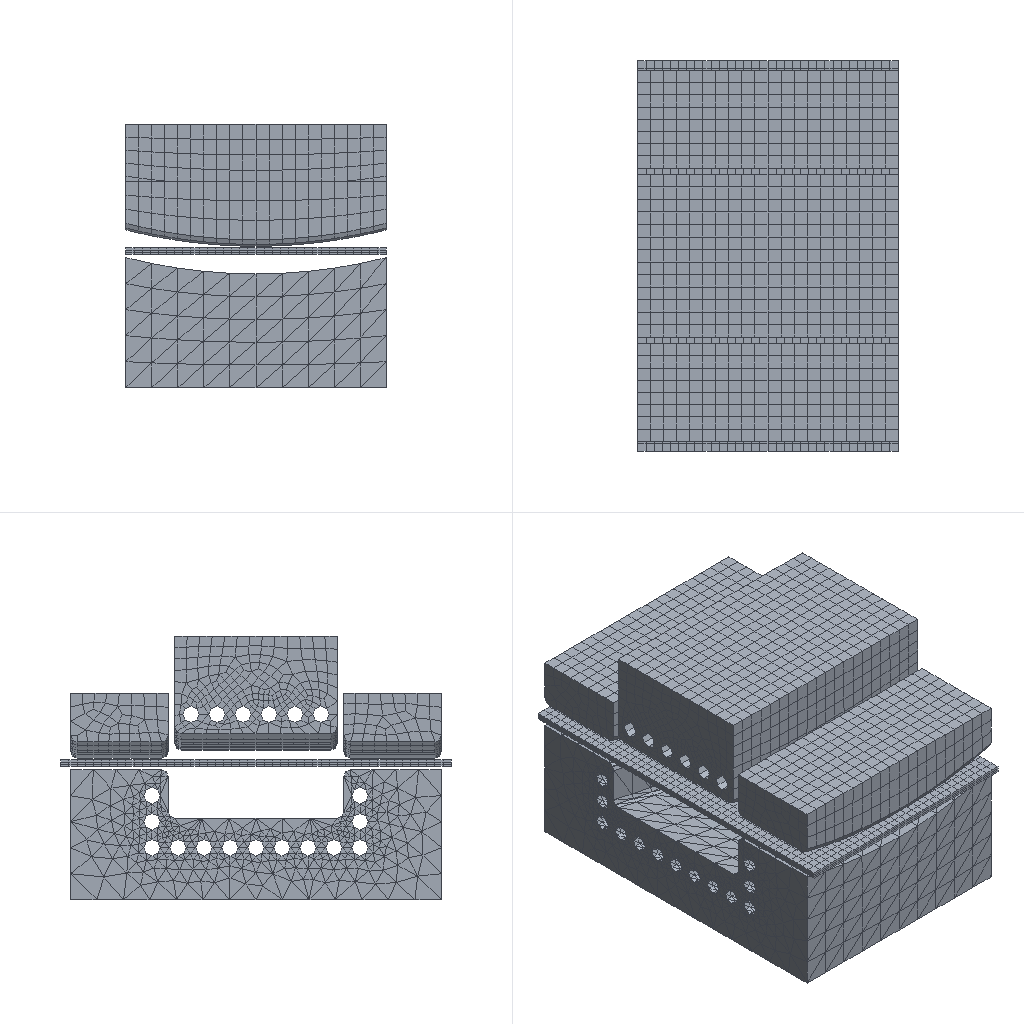Simulation study | abaqus
Set-up summary:
category,name,step,type,value,unit,region
solver,abaqus
solver,version,,,Abaqus/Explicit 2020
units,not stated in the deck,,not stated
analysis,deck,,dynamic temperature-displacement,dynamic temperature-displacement
load_step,Step-1,Step-1,dynamic temperature-displacement
load_step,requested,,,1
mesh,nodes,,,24140
mesh,elements,,,54890
element_type,C3D4,,solid,44042
element_type,C3D8R,,solid,6240
element_type,C3D8RT,,solid,4608
load,load commands in deck,,count,4
bc,support commands in deck,,count,15
material,MATERIAL-1,,in results
material,MATERIAL-RIGID,,in results
check,setup vs results,,match,"per instance, exact: element labels, types and connectivity; labels of the nodes the elements use; coordinates not compared"
Abaqus input file, long lists of numbers shortened:
*Heading
** Job name: Job-2 Model name: Model-1
** Generated by: Abaqus/CAE 2020
*Preprint, echo=NO, model=NO, history=NO, contact=NO
**
** PARTS
**
*Part, name=zhuangpeitu-1
*Node
      1,         -40.,          60.,           1.
      2,         -40.,         57.5,           1.
** (6466 more lines like these left out)
*Element, type=C3D8RT
   1,  197,  198,  247,  246,    1,    2,   51,   50
   2,  198,  199,  248,  247,    2,    3,   52,   51
** (4606 more lines like these left out)
*Nset, nset=Set-3, generate
    1,  6468,     1
*Elset, elset=Set-3, generate
    1,  4608,     1
*Nset, nset=tt, generate
    1,  6468,     1
** Section: Section-1
*Solid Section, elset=Set-3, material=Material-1
,
*End Part
**
*Part, name=zhuangpeitu-2
*Node
      1,         -40.,          32.,        -13.5
      2,         -40.,           8.,        -21.5
** (9669 more lines like these left out)
*Element, type=C3D4
    1, 5348, 5349, 5350, 5351
    2, 5348, 5352, 5349, 5351
** (44040 more lines like these left out)
*Nset, nset=Set-10, generate
    1,  9671,     1
*Elset, elset=Set-10, generate
     1,  44042,      1
** Section: Section-2
*Solid Section, elset=Set-10, material=Material-rigid
,
*End Part
**
*Part, name=zhuangpeitu-3
*Node
      1,         -40.,    18.232,    20.268
      2,         -40.,         17.5,         18.5
** (5689 more lines like these left out)
*Element, type=C3D8R
   1,  152,  155,  158,  257,  423,  426,  429,  528
   2,  135,   93,   48,   47,  406,  364,  319,  318
** (4598 more lines like these left out)
*Nset, nset=Set-2, generate
    1,  5691,     1
*Elset, elset=Set-2, generate
    1,  4600,     1
** Section: Section-2
*Solid Section, elset=Set-2, material=Material-rigid
,
*End Part
**
*Part, name=zhuangpeitu-4
*Node
      1,         -40.,          55.,          10.
      2,         -40.,          29.,          10.
** (1174 more lines like these left out)
*Element, type=C3D8R
  1,   22,   38,   37,   21,   78,   94,   93,   77
  2,    2,   33,    4,    3,   58,   89,   60,   59
** (838 more lines like these left out)
*Nset, nset=Set-2, generate
    1,  1176,     1
*Elset, elset=Set-2, generate
   1,  840,    1
** Section: Section-2
*Solid Section, elset=Set-2, material=Material-rigid
,
*End Part
**
*Part, name=zhuangpeitu-5
*Node
      1,         -40.,         -27.,          25.
      2,         -40.,         -27.,   12.064
** (1132 more lines like these left out)
*Element, type=C3D8R
  1,   54,   17,    4,   53,  108,   71,   58,  107
  2,   23,   37,   38,   24,   77,   91,   92,   78
** (798 more lines like these left out)
*Nset, nset=Set-2, generate
    1,  1134,     1
*Elset, elset=Set-2, generate
   1,  800,    1
** Section: Section-2
*Solid Section, elset=Set-2, material=Material-rigid
,
*End Part
**
**
** ASSEMBLY
**
*Assembly, name=Assembly
**
*Instance, name=zhuangpeitu-1-1, part=zhuangpeitu-1
*End Instance
**
*Instance, name=zhuangpeitu-2-1, part=zhuangpeitu-2
*End Instance
**
*Instance, name=zhuangpeitu-3-1, part=zhuangpeitu-3
          0.,           0.,         -1.5
*End Instance
**
*Instance, name=zhuangpeitu-4-1, part=zhuangpeitu-4
          0.,           0.,         -1.5
*End Instance
**
*Instance, name=zhuangpeitu-5-1, part=zhuangpeitu-5
          0.,           0.,         -1.5
*End Instance
**
*Node
      1,          40.,         -42.,         23.5
*Node
      2,          40.,          42.,         23.5
*Node
      3,          40.,           0.,          41.
*Node
      4,          40.,           0.,         -40.
*Nset, nset=Set-9, instance=zhuangpeitu-1-1, generate
    1,  6468,     1
*Nset, nset=Set-9, instance=zhuangpeitu-2-1, generate
    1,  9671,     1
*Nset, nset=Set-9, instance=zhuangpeitu-4-1, generate
    1,  1176,     1
*Nset, nset=Set-9, instance=zhuangpeitu-3-1, generate
    1,  5691,     1
*Nset, nset=Set-9, instance=zhuangpeitu-5-1, generate
    1,  1134,     1
*Elset, elset=Set-9, instance=zhuangpeitu-1-1, generate
    1,  4608,     1
*Elset, elset=Set-9, instance=zhuangpeitu-2-1, generate
     1,  44042,      1
*Elset, elset=Set-9, instance=zhuangpeitu-4-1, generate
   1,  840,    1
*Elset, elset=Set-9, instance=zhuangpeitu-3-1, generate
    1,  4600,     1
*Elset, elset=Set-9, instance=zhuangpeitu-5-1, generate
   1,  800,    1
*Nset, nset=Set-10
 1, 2
*Nset, nset=Set-11
 3,
*Nset, nset=Set-12
 4,
*Nset, nset=Set-13, instance=zhuangpeitu-1-1, generate
    1,  6468,     1
*Elset, elset=Set-13, instance=zhuangpeitu-1-1, generate
    1,  4608,     1
*Nset, nset=Set-14, instance=zhuangpeitu-1-1
    1,   49,   50,   98,   99,  147,  148,  196,  197,  245,  246,  294,  295,  343,  344,  392
  393,  441,  442,  490,  491,  539,  540,  588,  589,  637,  638,  686,  687,  735,  736,  784
** (15 more lines like these left out)
*Elset, elset=Set-14, instance=zhuangpeitu-1-1
    1,   48,   49,   96,   97,  144,  145,  192,  193,  240,  241,  288,  289,  336,  337,  384
  385,  432,  433,  480,  481,  528,  529,  576,  577,  624,  625,  672,  673,  720,  721,  768
** (10 more lines like these left out)
*Nset, nset=Set-15, instance=zhuangpeitu-1-1
    1,    2,    3,    4,    5,    6,    7,    8,    9,   10,   11,   12,   13,   14,   15,   16
   17,   18,   19,   20,   21,   22,   23,   24,   25,   26,   27,   28,   29,   30,   31,   32
** (23 more lines like these left out)
*Elset, elset=Set-15, instance=zhuangpeitu-1-1
    1,    2,    3,    4,    5,    6,    7,    8,    9,   10,   11,   12,   13,   14,   15,   16
   17,   18,   19,   20,   21,   22,   23,   24,   25,   26,   27,   28,   29,   30,   31,   32
** (16 more lines like these left out)
*Nset, nset=b_Set-1, instance=zhuangpeitu-3-1, generate
    1,  5691,     1
*Elset, elset=b_Set-1, instance=zhuangpeitu-3-1, generate
    1,  4600,     1
*Nset, nset=b_Set-3, instance=zhuangpeitu-5-1, generate
    1,  1134,     1
*Elset, elset=b_Set-3, instance=zhuangpeitu-5-1, generate
   1,  800,    1
*Nset, nset=b_Set-5, instance=zhuangpeitu-4-1, generate
    1,  1176,     1
*Elset, elset=b_Set-5, instance=zhuangpeitu-4-1, generate
   1,  840,    1
*Nset, nset=b_Set-7, instance=zhuangpeitu-2-1, generate
    1,  9671,     1
*Elset, elset=b_Set-7, instance=zhuangpeitu-2-1, generate
     1,  44042,      1
*Nset, nset=_PickedSet17, internal
 3,
*Nset, nset=_PickedSet19, internal
 1,
*Nset, nset=_PickedSet21, internal
 2,
*Nset, nset=_PickedSet23, internal
 4,
*Elset, elset=_Surf-7_S1, internal, instance=zhuangpeitu-1-1, generate
 4465,  4608,     1
*Elset, elset=_Surf-7_S4, internal, instance=zhuangpeitu-1-1, generate
   48,  4608,    48
*Elset, elset=_Surf-7_S2, internal, instance=zhuangpeitu-1-1, generate
   1,  144,    1
*Elset, elset=_Surf-7_S6, internal, instance=zhuangpeitu-1-1, generate
    1,  4561,    48
*Elset, elset=_Surf-7_S5, internal, instance=zhuangpeitu-1-1
   97,   98,   99,  100,  101,  102,  103,  104,  105,  106,  107,  108,  109,  110,  111,  112
  113,  114,  115,  116,  117,  118,  119,  120,  121,  122,  123,  124,  125,  126,  127,  128
** (94 more lines like these left out)
*Elset, elset=_Surf-7_S3, internal, instance=zhuangpeitu-1-1
    1,    2,    3,    4,    5,    6,    7,    8,    9,   10,   11,   12,   13,   14,   15,   16
   17,   18,   19,   20,   21,   22,   23,   24,   25,   26,   27,   28,   29,   30,   31,   32
** (94 more lines like these left out)
*Surface, type=ELEMENT, name=Surf-7
_Surf-7_S1, S1
_Surf-7_S4, S4
_Surf-7_S2, S2
_Surf-7_S6, S6
_Surf-7_S5, S5
_Surf-7_S3, S3
*Elset, elset=_Surf-8_S1, internal, instance=zhuangpeitu-1-1, generate
 4465,  4608,     1
*Elset, elset=_Surf-8_S2, internal, instance=zhuangpeitu-1-1, generate
   1,  144,    1
*Elset, elset=_Surf-8_S5, internal, instance=zhuangpeitu-1-1
   97,   98,   99,  100,  101,  102,  103,  104,  105,  106,  107,  108,  109,  110,  111,  112
  113,  114,  115,  116,  117,  118,  119,  120,  121,  122,  123,  124,  125,  126,  127,  128
** (94 more lines like these left out)
*Elset, elset=_Surf-8_S3, internal, instance=zhuangpeitu-1-1
    1,    2,    3,    4,    5,    6,    7,    8,    9,   10,   11,   12,   13,   14,   15,   16
   17,   18,   19,   20,   21,   22,   23,   24,   25,   26,   27,   28,   29,   30,   31,   32
** (94 more lines like these left out)
*Surface, type=ELEMENT, name=Surf-8
_Surf-8_S1, S1
_Surf-8_S2, S2
_Surf-8_S5, S5
_Surf-8_S3, S3
*Elset, elset=_m_Surf-1_S2, internal, instance=zhuangpeitu-4-1, generate
 799,  840,    1
*Elset, elset=_m_Surf-1_S3, internal, instance=zhuangpeitu-4-1
   5,   6,   8,   9,  11,  12,  21,  22,  23,  47,  48,  50,  51,  53,  54,  63
  64,  65,  89,  90,  92,  93,  95,  96, 105, 106, 107, 131, 132, 134, 135, 137
** (10 more lines like these left out)
*Elset, elset=_m_Surf-1_S5, internal, instance=zhuangpeitu-4-1
   2,  13,  15,  20,  32,  42,  44,  55,  57,  62,  74,  84,  86,  97,  99, 104
 116, 126, 128, 139, 141, 146, 158, 168, 170, 181, 183, 188, 200, 210, 212, 223
** (6 more lines like these left out)
*Elset, elset=_m_Surf-1_S4, internal, instance=zhuangpeitu-4-1, generate
  25,  823,   42
*Elset, elset=_m_Surf-1_S1, internal, instance=zhuangpeitu-4-1, generate
  1,  42,   1
*Elset, elset=_m_Surf-1_S6, internal, instance=zhuangpeitu-4-1
   2,  21,  44,  63,  86, 105, 128, 147, 170, 189, 212, 231, 254, 273, 296, 315
 338, 357, 380, 399, 422, 441, 464, 483, 506, 525, 548, 567, 590, 609, 632, 651
** (1 more lines like these left out)
*Surface, type=ELEMENT, name=m_Surf-1
_m_Surf-1_S2, S2
_m_Surf-1_S3, S3
_m_Surf-1_S4, S4
_m_Surf-1_S6, S6
_m_Surf-1_S5, S5
_m_Surf-1_S1, S1
*Elset, elset=_m_Surf-3_S1, internal, instance=zhuangpeitu-3-1, generate
   1,  230,    1
*Elset, elset=_m_Surf-3_S3, internal, instance=zhuangpeitu-3-1
    3,    8,   19,   28,   44,   48,   56,   61,  100,  113,  233,  238,  249,  258,  274,  278
  286,  291,  330,  343,  463,  468,  479,  488,  504,  508,  516,  521,  560,  573,  693,  698
** (11 more lines like these left out)
*Elset, elset=_m_Surf-3_S6, internal, instance=zhuangpeitu-3-1
   13,   15,   26,   30,   93,  197,  243,  245,  256,  260,  323,  427,  473,  475,  486,  490
  553,  657,  703,  705,  716,  720,  783,  887,  933,  935,  946,  950, 1013, 1117, 1163, 1165
** (6 more lines like these left out)
*Elset, elset=_m_Surf-3_S5, internal, instance=zhuangpeitu-3-1
   40,   45,   52,   59,   65,   80,  120,  270,  275,  282,  289,  295,  310,  350,  500,  505
  512,  519,  525,  540,  580,  730,  735,  742,  749,  755,  770,  810,  960,  965,  972,  979
** (7 more lines like these left out)
*Elset, elset=_m_Surf-3_S4, internal, instance=zhuangpeitu-3-1
   51,   69,   91,  105,  113,  119,  165,  209,  281,  299,  321,  335,  343,  349,  395,  439
  511,  529,  551,  565,  573,  579,  625,  669,  741,  759,  781,  795,  803,  809,  855,  899
** (8 more lines like these left out)
*Elset, elset=_m_Surf-3_S2, internal, instance=zhuangpeitu-3-1, generate
 4371,  4600,     1
*Surface, type=ELEMENT, name=m_Surf-3
_m_Surf-3_S1, S1
_m_Surf-3_S3, S3
_m_Surf-3_S6, S6
_m_Surf-3_S4, S4
_m_Surf-3_S2, S2
_m_Surf-3_S5, S5
*Elset, elset=_m_Surf-4_S2, internal, instance=zhuangpeitu-5-1, generate
 761,  800,    1
*Elset, elset=_m_Surf-4_S4, internal, instance=zhuangpeitu-5-1
   1,   6,  19,  23,  40,  41,  46,  59,  63,  80,  81,  86,  99, 103, 120, 121
 126, 139, 143, 160, 161, 166, 179, 183, 200, 201, 206, 219, 223, 240, 241, 246
** (5 more lines like these left out)
*Elset, elset=_m_Surf-4_S5, internal, instance=zhuangpeitu-5-1
   4,   5,  11,  21,  22,  44,  45,  51,  61,  62,  84,  85,  91, 101, 102, 124
 125, 131, 141, 142, 164, 165, 171, 181, 182, 204, 205, 211, 221, 222, 244, 245
** (5 more lines like these left out)
*Elset, elset=_m_Surf-4_S3, internal, instance=zhuangpeitu-5-1
   9,  10,  20,  40,  49,  50,  60,  80,  89,  90, 100, 120, 129, 130, 140, 160
 169, 170, 180, 200, 209, 210, 220, 240, 249, 250, 260, 280, 289, 290, 300, 320
** (3 more lines like these left out)
*Elset, elset=_m_Surf-4_S1, internal, instance=zhuangpeitu-5-1, generate
  1,  40,   1
*Elset, elset=_m_Surf-4_S6, internal, instance=zhuangpeitu-5-1
   5,   7,  18,  25,  45,  47,  58,  65,  85,  87,  98, 105, 125, 127, 138, 145
 165, 167, 178, 185, 205, 207, 218, 225, 245, 247, 258, 265, 285, 287, 298, 305
** (3 more lines like these left out)
*Surface, type=ELEMENT, name=m_Surf-4
_m_Surf-4_S2, S2
_m_Surf-4_S4, S4
_m_Surf-4_S6, S6
_m_Surf-4_S5, S5
_m_Surf-4_S3, S3
_m_Surf-4_S1, S1
*Elset, elset=_m_Surf-5_S3, internal, instance=zhuangpeitu-2-1
   276,   802,  3169,  4184,  4667,  6453,  6546,  6793,  6988,  7217,  7271,  7348,  7421,  7458,  7502,  7774
  8108,  8463,  8669,  8685,  8957,  9390,  9666,  9728,  9967, 10313, 10601, 10805, 11017, 11051, 11349, 11584
** (18 more lines like these left out)
*Elset, elset=_m_Surf-5_S4, internal, instance=zhuangpeitu-2-1
   119,   144,  1161,  1215,  1280,  1634,  1664,  1817,  1826,  1983,  2033,  2214,  2297,  2298,  2641,  3411
  3712,  7867, 11115, 11673, 12007, 13240, 13247, 13690, 15522, 17188, 18439, 19206, 19503, 20601, 21223, 21258
** (3 more lines like these left out)
*Elset, elset=_m_Surf-5_S2, internal, instance=zhuangpeitu-2-1
  1296,  1935,  2209,  2912,  3250,  6296,  6984,  7028,  7259, 10016, 11114, 11128, 12396, 12407, 14166, 14215
 14366, 14610, 18423, 18885, 18939, 19107, 19283, 19302, 19884, 20023, 20279, 21183, 22702, 22775, 22940, 22971
** (2 more lines like these left out)
*Elset, elset=_m_Surf-5_S1, internal, instance=zhuangpeitu-2-1
  1607,  3198,  6316,  7626,  7819,  9232,  9288, 12307, 17285, 17707, 18847, 19067, 19093, 19704, 20117, 20640
 21890, 23832, 23847, 23929, 24016, 27824, 28081, 28517, 29268, 29512, 30579, 30783, 31315, 33710, 34848, 35888
** (1 more lines like these left out)
*Surface, type=ELEMENT, name=m_Surf-5
_m_Surf-5_S3, S3
_m_Surf-5_S4, S4
_m_Surf-5_S2, S2
_m_Surf-5_S1, S1
*Elset, elset=_s_Surf-1_S5, internal, instance=zhuangpeitu-1-1
   97,   98,   99,  100,  101,  102,  103,  104,  105,  106,  107,  108,  109,  110,  111,  112
  113,  114,  115,  116,  117,  118,  119,  120,  121,  122,  123,  124,  125,  126,  127,  128
** (94 more lines like these left out)
*Surface, type=ELEMENT, name=s_Surf-1
_s_Surf-1_S5, S5
*Elset, elset=_s_Surf-5_S3, internal, instance=zhuangpeitu-1-1
    1,    2,    3,    4,    5,    6,    7,    8,    9,   10,   11,   12,   13,   14,   15,   16
   17,   18,   19,   20,   21,   22,   23,   24,   25,   26,   27,   28,   29,   30,   31,   32
** (94 more lines like these left out)
*Surface, type=ELEMENT, name=s_Surf-5
_s_Surf-5_S3, S3
*Surface, type=NODE, name=zhuangpeitu-1-1_tt_CNS_, internal
zhuangpeitu-1-1.tt, 1.
** Constraint: Constraint-1
*Rigid Body, ref node=_PickedSet17, elset=b_Set-1, position=CENTER OF MASS
** Constraint: Constraint-2
*Rigid Body, ref node=_PickedSet19, elset=b_Set-3, position=CENTER OF MASS
** Constraint: Constraint-3
*Rigid Body, ref node=_PickedSet21, elset=b_Set-5, position=CENTER OF MASS
** Constraint: Constraint-4
*Rigid Body, ref node=_PickedSet23, elset=b_Set-7, position=CENTER OF MASS
*End Assembly
**
** MATERIALS
**
*Material, name=Material-1
*Conductivity
 30.7, 20.
 31.1,100.
  30.,200.
 27.5,300.
 21.7,400.
 23.6,600.
 25.6,800.
*Density
 7.8e-09,
*Elastic
212000., 0.284,   20.
207000., 0.286,  100.
199000., 0.289,  200.
193000., 0.293,  300.
166000., 0.298,  400.
150000.,  0.31,  600.
134000., 0.325,  800.
*Plastic, hardening=JOHNSON COOK
714.,  563., 0.518, 0.698, 1500.,   20.
*Rate Dependent, type=JOHNSON COOK
 0.037,1.
*Specific Heat
 4.44e+08, 20.
 4.87e+08,100.
  5.2e+08,200.
 5.44e+08,300.
 5.61e+08,400.
 5.81e+08,600.
  5.9e+08,800.
*Material, name=Material-rigid
*Density
 7.8e-09,
*Elastic
212000., 0.284,   20.
207000., 0.286,  100.
199000., 0.289,  200.
193000., 0.293,  300.
166000., 0.298,  400.
150000.,  0.31,  600.
134000., 0.325,  800.
**
** INTERACTION PROPERTIES
**
*Surface Interaction, name=IntProp-1
*Friction
 0.6,
*Surface Behavior, pressure-overclosure=HARD
**
** PHYSICAL CONSTANTS
**
*Physical Constants, absolute zero=-273., stefan boltzmann=5.67e-08
**
** BOUNDARY CONDITIONS
**
** Name: BC-5 Type: 位移/转角
*Boundary
Set-15, 1, 1
Set-15, 2, 2
**
** PREDEFINED FIELDS
**
** Name: Predefined Field-1   Type: Temperature
*Initial Conditions, type=TEMPERATURE
Set-13, 1200.
** ----------------------------------------------------------------
**
** STEP: Step-1
**
*Step, name=Step-1, nlgeom=YES
*Dynamic Temperature-displacement, Explicit
, 0.1
*Bulk Viscosity
0.06, 1.2
** Mass Scaling: Semi-Automatic
**               Whole Model
*Fixed Mass Scaling, factor=500.
**
** BOUNDARY CONDITIONS
**
** Name: BC-1 Type: 速度/角速度
*Boundary, type=VELOCITY
Set-10, 1, 1
Set-10, 2, 2
Set-10, 3, 3, -65.
Set-10, 4, 4
Set-10, 5, 5
Set-10, 6, 6
** Name: BC-3 Type: 对称/反对称/完全固定
*Boundary
Set-12, ENCASTRE
** Name: [REDACTED] : Velocity/Angular velocity
*Boundary, type=VELOCITY
Set-11, 1, 1
Set-11, 2, 2
Set-11, 3, 3, -240.
Set-11, 4, 4
Set-11, 5, 5
Set-11, 6, 6
**
** INTERACTIONS
**
** Interaction: Int-1
*Contact Pair, interaction=IntProp-1, mechanical constraint=KINEMATIC, cpset=Int-1
m_Surf-1, zhuangpeitu-1-1_tt_CNS_
** Interaction: Int-1-Copy
*Contact Pair, interaction=IntProp-1, mechanical constraint=KINEMATIC, cpset=Int-1-Copy
m_Surf-3, zhuangpeitu-1-1_tt_CNS_
** Interaction: Int-1-Copy2
*Contact Pair, interaction=IntProp-1, mechanical constraint=KINEMATIC, cpset=Int-1-Copy2
m_Surf-4, zhuangpeitu-1-1_tt_CNS_
** Interaction: Int-2
*Contact Pair, interaction=IntProp-1, mechanical constraint=KINEMATIC, cpset=Int-2
m_Surf-5, zhuangpeitu-1-1_tt_CNS_
** Interaction: Int-5
*Sradiate
Surf-7, R, 20., 0.8
** Interaction: Int-6
*Sfilm
Surf-8, F, 20., 0.5
**
** OUTPUT REQUESTS
**
*Restart, write, number interval=1, time marks=NO
**
** FIELD OUTPUT: F-Output-1
**
*Output, field, number interval=100
*Node Output, exterior
A, NT, RF, RFL, U, V
*Element Output, exterior, directions=YES
E, HFL, LE, MISES, PE, PEEQ, PEEQVAVG, PEVAVG, S, SVAVG, TEMP
*Contact Output
CSTRESS,
**
** HISTORY OUTPUT: H-Output-1
**
*Output, history, variable=PRESELECT
*End Step
Results summary:
result,step,Step-1,completed,increments=56180 time=0.1/0.1
result,analysis,,,"dynamic temperature-displacement, explict"
result,last_loadstep,,,1
result,primary field,,,"U, NT11"
result,reaction total,,FX,-10.186,model units
result,reaction total,,FY,-8.472,model units
result,reaction total,,FZ,0.0,model units